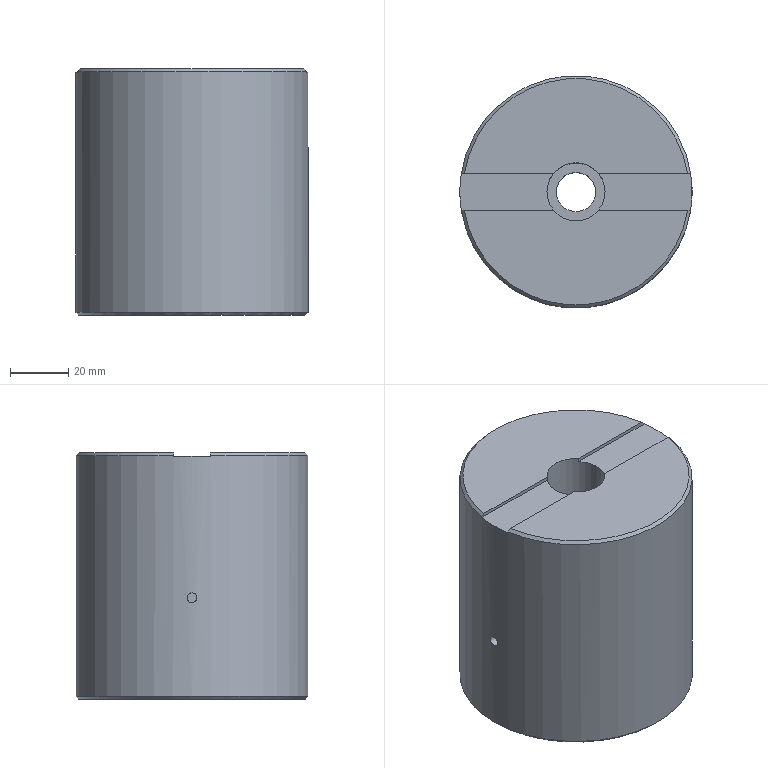Part | STEP file | 008_id4122_x_t | 1 solid | 18 faces | box 80 x 80 x 85 mm | volume 404311 mm3 | plane 11 | cylinder 4 | cone 3 | commonest cylinder face diameters 3.4 x1 13.509 x1 20.008 x1 80 x1
STEP:
#1=CARTESIAN_POINT('',(2359.705,-548.65,5.));
#2=VERTEX_POINT('',#1);
#3=CARTESIAN_POINT('',(2328.956,-548.65,5.));
#4=VERTEX_POINT('',#3);
#5=CARTESIAN_POINT('',(2415.936,-548.65,5.));
#6=DIRECTION('',(-1.,0.,0.));
#7=VECTOR('',#6,1.);
#8=LINE('',#5,#7);
#9=EDGE_CURVE('',#2,#4,#8,.T.);
#10=ORIENTED_EDGE('',*,*,#9,.F.);
#11=CARTESIAN_POINT('',(2375.166,-548.65,5.));
#12=VERTEX_POINT('',#11);
#13=CARTESIAN_POINT('',(2367.435,-555.,5.));
#14=DIRECTION('',(0.,0.,-1.));
#15=DIRECTION('',(1.,0.,0.));
#16=AXIS2_PLACEMENT_3D('',#13,#14,#15);
#17=CIRCLE('',#16,10.004);
#18=EDGE_CURVE('',#2,#12,#17,.T.);
#19=ORIENTED_EDGE('',*,*,#18,.T.);
#20=CARTESIAN_POINT('',(2405.915,-548.65,5.));
#21=VERTEX_POINT('',#20);
#22=CARTESIAN_POINT('',(2415.936,-548.65,5.));
#23=DIRECTION('',(-1.,0.,0.));
#24=VECTOR('',#23,1.);
#25=LINE('',#22,#24);
#26=EDGE_CURVE('',#21,#12,#25,.T.);
#27=ORIENTED_EDGE('',*,*,#26,.F.);
#28=CARTESIAN_POINT('',(2367.435,-555.,5.));
#29=DIRECTION('',(0.,0.,-1.));
#30=DIRECTION('',(-1.,0.,0.));
#31=AXIS2_PLACEMENT_3D('',#28,#29,#30);
#32=CIRCLE('',#31,39.);
#33=EDGE_CURVE('',#4,#21,#32,.T.);
#34=ORIENTED_EDGE('',*,*,#33,.F.);
#35=EDGE_LOOP('',(#10,#19,#27,#34));
#36=FACE_OUTER_BOUND('',#35,.T.);
#37=CARTESIAN_POINT('',(2367.435,-555.,5.));
#38=DIRECTION('',(0.,0.,1.));
#39=DIRECTION('',(-1.,0.,0.));
#40=AXIS2_PLACEMENT_3D('',#37,#38,#39);
#41=PLANE('',#40);
#42=ADVANCED_FACE('',(#36),#41,.T.);
#43=CARTESIAN_POINT('',(2405.915,-561.35,5.));
#44=VERTEX_POINT('',#43);
#45=CARTESIAN_POINT('',(2375.166,-561.35,5.));
#46=VERTEX_POINT('',#45);
#47=CARTESIAN_POINT('',(2415.936,-561.35,5.));
#48=DIRECTION('',(-1.,0.,0.));
#49=VECTOR('',#48,1.);
#50=LINE('',#47,#49);
#51=EDGE_CURVE('',#44,#46,#50,.T.);
#52=ORIENTED_EDGE('',*,*,#51,.T.);
#53=CARTESIAN_POINT('',(2359.705,-561.35,5.));
#54=VERTEX_POINT('',#53);
#55=CARTESIAN_POINT('',(2367.435,-555.,5.));
#56=DIRECTION('',(0.,0.,-1.));
#57=DIRECTION('',(1.,0.,0.));
#58=AXIS2_PLACEMENT_3D('',#55,#56,#57);
#59=CIRCLE('',#58,10.004);
#60=EDGE_CURVE('',#46,#54,#59,.T.);
#61=ORIENTED_EDGE('',*,*,#60,.T.);
#62=CARTESIAN_POINT('',(2328.956,-561.35,5.));
#63=VERTEX_POINT('',#62);
#64=CARTESIAN_POINT('',(2415.936,-561.35,5.));
#65=DIRECTION('',(-1.,0.,0.));
#66=VECTOR('',#65,1.);
#67=LINE('',#64,#66);
#68=EDGE_CURVE('',#54,#63,#67,.T.);
#69=ORIENTED_EDGE('',*,*,#68,.T.);
#70=CARTESIAN_POINT('',(2367.435,-555.,5.));
#71=DIRECTION('',(0.,0.,-1.));
#72=DIRECTION('',(-1.,0.,0.));
#73=AXIS2_PLACEMENT_3D('',#70,#71,#72);
#74=CIRCLE('',#73,39.);
#75=EDGE_CURVE('',#44,#63,#74,.T.);
#76=ORIENTED_EDGE('',*,*,#75,.F.);
#77=EDGE_LOOP('',(#52,#61,#69,#76));
#78=FACE_OUTER_BOUND('',#77,.T.);
#79=CARTESIAN_POINT('',(2367.435,-555.,5.));
#80=DIRECTION('',(0.,0.,1.));
#81=DIRECTION('',(-1.,0.,0.));
#82=AXIS2_PLACEMENT_3D('',#79,#80,#81);
#83=PLANE('',#82);
#84=ADVANCED_FACE('',(#78),#83,.T.);
#85=CARTESIAN_POINT('',(2327.435,-555.,-79.));
#86=VERTEX_POINT('',#85);
#87=CARTESIAN_POINT('',(2367.435,-555.,-79.));
#88=DIRECTION('',(0.,0.,-1.));
#89=DIRECTION('',(-1.,0.,0.));
#90=AXIS2_PLACEMENT_3D('',#87,#88,#89);
#91=CIRCLE('',#90,40.);
#92=EDGE_CURVE('',#86,#86,#91,.T.);
#93=ORIENTED_EDGE('',*,*,#92,.F.);
#94=EDGE_LOOP('',(#93));
#95=FACE_BOUND('',#94,.T.);
#96=CARTESIAN_POINT('',(2406.928,-548.65,3.73));
#97=VERTEX_POINT('',#96);
#98=CARTESIAN_POINT('',(2406.928,-548.65,4.));
#99=VERTEX_POINT('',#98);
#100=CARTESIAN_POINT('',(2406.928,-548.65,-80.));
#101=DIRECTION('',(0.,0.,1.));
#102=VECTOR('',#101,1.);
#103=LINE('',#100,#102);
#104=EDGE_CURVE('',#97,#99,#103,.T.);
#105=ORIENTED_EDGE('',*,*,#104,.F.);
#106=CARTESIAN_POINT('',(2406.928,-561.35,3.73));
#107=VERTEX_POINT('',#106);
#108=CARTESIAN_POINT('',(2367.435,-555.,3.73));
#109=DIRECTION('',(0.,0.,1.));
#110=DIRECTION('',(0.,-1.,0.));
#111=AXIS2_PLACEMENT_3D('',#108,#109,#110);
#112=CIRCLE('',#111,40.);
#113=EDGE_CURVE('',#107,#97,#112,.T.);
#114=ORIENTED_EDGE('',*,*,#113,.F.);
#115=CARTESIAN_POINT('',(2406.928,-561.35,4.));
#116=VERTEX_POINT('',#115);
#117=CARTESIAN_POINT('',(2406.928,-561.35,-80.));
#118=DIRECTION('',(0.,0.,-1.));
#119=VECTOR('',#118,1.);
#120=LINE('',#117,#119);
#121=EDGE_CURVE('',#116,#107,#120,.T.);
#122=ORIENTED_EDGE('',*,*,#121,.F.);
#123=CARTESIAN_POINT('',(2327.942,-561.35,4.));
#124=VERTEX_POINT('',#123);
#125=CARTESIAN_POINT('',(2367.435,-555.,4.));
#126=DIRECTION('',(0.,0.,1.));
#127=DIRECTION('',(-1.,0.,0.));
#128=AXIS2_PLACEMENT_3D('',#125,#126,#127);
#129=CIRCLE('',#128,40.);
#130=EDGE_CURVE('',#124,#116,#129,.T.);
#131=ORIENTED_EDGE('',*,*,#130,.F.);
#132=CARTESIAN_POINT('',(2327.942,-561.35,3.73));
#133=VERTEX_POINT('',#132);
#134=CARTESIAN_POINT('',(2327.942,-561.35,-80.));
#135=DIRECTION('',(0.,0.,1.));
#136=VECTOR('',#135,1.);
#137=LINE('',#134,#136);
#138=EDGE_CURVE('',#133,#124,#137,.T.);
#139=ORIENTED_EDGE('',*,*,#138,.F.);
#140=CARTESIAN_POINT('',(2327.942,-548.65,3.73));
#141=VERTEX_POINT('',#140);
#142=CARTESIAN_POINT('',(2367.435,-555.,3.73));
#143=DIRECTION('',(0.,0.,1.));
#144=DIRECTION('',(0.,-1.,0.));
#145=AXIS2_PLACEMENT_3D('',#142,#143,#144);
#146=CIRCLE('',#145,40.);
#147=EDGE_CURVE('',#141,#133,#146,.T.);
#148=ORIENTED_EDGE('',*,*,#147,.F.);
#149=CARTESIAN_POINT('',(2327.942,-548.65,4.));
#150=VERTEX_POINT('',#149);
#151=CARTESIAN_POINT('',(2327.942,-548.65,-80.));
#152=DIRECTION('',(0.,0.,-1.));
#153=VECTOR('',#152,1.);
#154=LINE('',#151,#153);
#155=EDGE_CURVE('',#150,#141,#154,.T.);
#156=ORIENTED_EDGE('',*,*,#155,.F.);
#157=CARTESIAN_POINT('',(2367.435,-555.,4.));
#158=DIRECTION('',(0.,0.,1.));
#159=DIRECTION('',(-1.,0.,0.));
#160=AXIS2_PLACEMENT_3D('',#157,#158,#159);
#161=CIRCLE('',#160,40.);
#162=EDGE_CURVE('',#99,#150,#161,.T.);
#163=ORIENTED_EDGE('',*,*,#162,.F.);
#164=EDGE_LOOP('',(#105,#114,#122,#131,#139,#148,#156,#163));
#165=FACE_BOUND('',#164,.T.);
#166=CARTESIAN_POINT('',(2327.436,-555.182,-43.31));
#167=VERTEX_POINT('',#166);
#168=CARTESIAN_POINT('',(2327.436,-555.182,-43.31));
#169=CARTESIAN_POINT('',(2327.435,-554.993,-43.289));
#170=CARTESIAN_POINT('',(2327.435,-554.798,-43.301));
#171=CARTESIAN_POINT('',(2327.437,-554.613,-43.345));
#172=CARTESIAN_POINT('',(2327.439,-554.427,-43.388));
#173=CARTESIAN_POINT('',(2327.442,-554.247,-43.464));
#174=CARTESIAN_POINT('',(2327.446,-554.087,-43.566));
#175=CARTESIAN_POINT('',(2327.449,-553.926,-43.668));
#176=CARTESIAN_POINT('',(2327.454,-553.781,-43.799));
#177=CARTESIAN_POINT('',(2327.458,-553.664,-43.949));
#178=CARTESIAN_POINT('',(2327.461,-553.546,-44.099));
#179=CARTESIAN_POINT('',(2327.465,-553.453,-44.271));
#180=CARTESIAN_POINT('',(2327.468,-553.391,-44.451));
#181=CARTESIAN_POINT('',(2327.47,-553.33,-44.631));
#182=CARTESIAN_POINT('',(2327.471,-553.298,-44.824));
#183=CARTESIAN_POINT('',(2327.471,-553.3,-45.014));
#184=CARTESIAN_POINT('',(2327.471,-553.302,-45.204));
#185=CARTESIAN_POINT('',(2327.47,-553.336,-45.397));
#186=CARTESIAN_POINT('',(2327.467,-553.4,-45.576));
#187=CARTESIAN_POINT('',(2327.465,-553.465,-45.755));
#188=CARTESIAN_POINT('',(2327.461,-553.561,-45.925));
#189=CARTESIAN_POINT('',(2327.457,-553.681,-46.072));
#190=CARTESIAN_POINT('',(2327.453,-553.801,-46.22));
#191=CARTESIAN_POINT('',(2327.449,-553.948,-46.349));
#192=CARTESIAN_POINT('',(2327.445,-554.11,-46.448));
#193=CARTESIAN_POINT('',(2327.442,-554.272,-46.548));
#194=CARTESIAN_POINT('',(2327.439,-554.454,-46.621));
#195=CARTESIAN_POINT('',(2327.437,-554.64,-46.661));
#196=CARTESIAN_POINT('',(2327.435,-554.826,-46.702));
#197=CARTESIAN_POINT('',(2327.435,-555.021,-46.71));
#198=CARTESIAN_POINT('',(2327.436,-555.21,-46.687));
#199=CARTESIAN_POINT('',(2327.437,-555.399,-46.664));
#200=CARTESIAN_POINT('',(2327.439,-555.586,-46.607));
#201=CARTESIAN_POINT('',(2327.442,-555.756,-46.523));
#202=CARTESIAN_POINT('',(2327.446,-555.926,-46.438));
#203=CARTESIAN_POINT('',(2327.45,-556.084,-46.323));
#204=CARTESIAN_POINT('',(2327.454,-556.217,-46.187));
#205=CARTESIAN_POINT('',(2327.458,-556.35,-46.051));
#206=CARTESIAN_POINT('',(2327.462,-556.461,-45.89));
#207=CARTESIAN_POINT('',(2327.465,-556.541,-45.717));
#208=CARTESIAN_POINT('',(2327.468,-556.622,-45.545));
#209=CARTESIAN_POINT('',(2327.47,-556.673,-45.356));
#210=CARTESIAN_POINT('',(2327.471,-556.692,-45.166));
#211=CARTESIAN_POINT('',(2327.472,-556.71,-44.977));
#212=CARTESIAN_POINT('',(2327.471,-556.697,-44.782));
#213=CARTESIAN_POINT('',(2327.469,-556.652,-44.597));
#214=CARTESIAN_POINT('',(2327.467,-556.607,-44.413));
#215=CARTESIAN_POINT('',(2327.464,-556.529,-44.233));
#216=CARTESIAN_POINT('',(2327.461,-556.425,-44.074));
#217=CARTESIAN_POINT('',(2327.457,-556.322,-43.914));
#218=CARTESIAN_POINT('',(2327.453,-556.189,-43.77));
#219=CARTESIAN_POINT('',(2327.449,-556.039,-43.654));
#220=CARTESIAN_POINT('',(2327.445,-555.888,-43.538));
#221=CARTESIAN_POINT('',(2327.441,-555.715,-43.446));
#222=CARTESIAN_POINT('',(2327.439,-555.535,-43.386));
#223=CARTESIAN_POINT('',(2327.437,-555.42,-43.348));
#224=CARTESIAN_POINT('',(2327.436,-555.301,-43.323));
#225=CARTESIAN_POINT('',(2327.436,-555.182,-43.31));
#226=B_SPLINE_CURVE_WITH_KNOTS('',3,(#168,#169,#170,#171,#172,#173,#174,#175,#176,#177,#178,#179,#180,#181,#182,#183,#184,#185,#186,#187,#188,#189,#190,#191,#192,#193,#194,#195,#196,#197,#198,#199,#200,#201,#202,#203,#204,#205,#206,#207,#208,#209,#210,#211,#212,#213,#214,#215,#216,#217,#218,#219,#220,#221,#222,#223,#224,#225),.UNSPECIFIED.,.T.,.F.,(1,3,3,3,3,3,3,3,3,3,3,3,3,3,3,3,3,3,3,3,3,1),(-0.03366,0.,0.05366,0.1073,0.161,0.2147,0.2684,0.3221,0.3757,0.4295,0.4832,0.5369,0.5905,0.6442,0.6979,0.7516,0.8053,0.8589,0.9126,0.9663,1.,1.054),.UNSPECIFIED.);
#227=EDGE_CURVE('',#167,#167,#226,.T.);
#228=ORIENTED_EDGE('',*,*,#227,.F.);
#229=EDGE_LOOP('',(#228));
#230=FACE_BOUND('',#229,.T.);
#231=CARTESIAN_POINT('',(2367.435,-555.,-80.));
#232=DIRECTION('',(0.,0.,1.));
#233=DIRECTION('',(-1.,0.,0.));
#234=AXIS2_PLACEMENT_3D('',#231,#232,#233);
#235=CYLINDRICAL_SURFACE('',#234,40.);
#236=ADVANCED_FACE('',(#95,#165,#230),#235,.T.);
#237=CARTESIAN_POINT('',(2374.19,-555.,-80.));
#238=VERTEX_POINT('',#237);
#239=CARTESIAN_POINT('',(2367.435,-555.,-80.));
#240=DIRECTION('',(0.,0.,1.));
#241=DIRECTION('',(1.,0.,0.));
#242=AXIS2_PLACEMENT_3D('',#239,#240,#241);
#243=CIRCLE('',#242,6.755);
#244=EDGE_CURVE('',#238,#238,#243,.T.);
#245=ORIENTED_EDGE('',*,*,#244,.T.);
#246=EDGE_LOOP('',(#245));
#247=FACE_BOUND('',#246,.T.);
#248=CARTESIAN_POINT('',(2328.435,-555.,-80.));
#249=VERTEX_POINT('',#248);
#250=CARTESIAN_POINT('',(2367.435,-555.,-80.));
#251=DIRECTION('',(0.,0.,1.));
#252=DIRECTION('',(-1.,0.,0.));
#253=AXIS2_PLACEMENT_3D('',#250,#251,#252);
#254=CIRCLE('',#253,39.);
#255=EDGE_CURVE('',#249,#249,#254,.T.);
#256=ORIENTED_EDGE('',*,*,#255,.F.);
#257=EDGE_LOOP('',(#256));
#258=FACE_BOUND('',#257,.T.);
#259=CARTESIAN_POINT('',(2367.435,-555.,-80.));
#260=DIRECTION('',(0.,0.,1.));
#261=DIRECTION('',(-1.,0.,0.));
#262=AXIS2_PLACEMENT_3D('',#259,#260,#261);
#263=PLANE('',#262);
#264=ADVANCED_FACE('',(#247,#258),#263,.F.);
#265=CARTESIAN_POINT('',(2375.166,-548.65,3.73));
#266=VERTEX_POINT('',#265);
#267=CARTESIAN_POINT('',(2375.166,-548.65,5.));
#268=DIRECTION('',(0.,0.,1.));
#269=VECTOR('',#268,1.);
#270=LINE('',#267,#269);
#271=EDGE_CURVE('',#266,#12,#270,.T.);
#272=ORIENTED_EDGE('',*,*,#271,.F.);
#273=CARTESIAN_POINT('',(2415.936,-548.65,3.73));
#274=DIRECTION('',(-1.,0.,0.));
#275=VECTOR('',#274,1.);
#276=LINE('',#273,#275);
#277=EDGE_CURVE('',#97,#266,#276,.T.);
#278=ORIENTED_EDGE('',*,*,#277,.F.);
#279=ORIENTED_EDGE('',*,*,#104,.T.);
#280=CARTESIAN_POINT('',(2405.915,-548.65,5.));
#281=CARTESIAN_POINT('',(2406.253,-548.65,4.667));
#282=CARTESIAN_POINT('',(2406.59,-548.65,4.333));
#283=CARTESIAN_POINT('',(2406.928,-548.65,4.));
#284=B_SPLINE_CURVE_WITH_KNOTS('',3,(#280,#281,#282,#283),.UNSPECIFIED.,.F.,.F.,(4,4),(0.,1.),.UNSPECIFIED.);
#285=EDGE_CURVE('',#21,#99,#284,.T.);
#286=ORIENTED_EDGE('',*,*,#285,.F.);
#287=ORIENTED_EDGE('',*,*,#26,.T.);
#288=EDGE_LOOP('',(#272,#278,#279,#286,#287));
#289=FACE_OUTER_BOUND('',#288,.T.);
#290=CARTESIAN_POINT('',(2415.936,-548.65,5.));
#291=DIRECTION('',(0.,-1.,0.));
#292=DIRECTION('',(0.,0.,-1.));
#293=AXIS2_PLACEMENT_3D('',#290,#291,#292);
#294=PLANE('',#293);
#295=ADVANCED_FACE('',(#289),#294,.T.);
#296=CARTESIAN_POINT('',(2375.166,-561.35,3.73));
#297=VERTEX_POINT('',#296);
#298=CARTESIAN_POINT('',(2367.435,-555.,3.73));
#299=DIRECTION('',(0.,0.,1.));
#300=DIRECTION('',(0.,-1.,0.));
#301=AXIS2_PLACEMENT_3D('',#298,#299,#300);
#302=CIRCLE('',#301,10.004);
#303=EDGE_CURVE('',#297,#266,#302,.T.);
#304=ORIENTED_EDGE('',*,*,#303,.F.);
#305=CARTESIAN_POINT('',(2415.936,-561.35,3.73));
#306=DIRECTION('',(-1.,0.,0.));
#307=VECTOR('',#306,1.);
#308=LINE('',#305,#307);
#309=EDGE_CURVE('',#107,#297,#308,.T.);
#310=ORIENTED_EDGE('',*,*,#309,.F.);
#311=ORIENTED_EDGE('',*,*,#113,.T.);
#312=ORIENTED_EDGE('',*,*,#277,.T.);
#313=EDGE_LOOP('',(#304,#310,#311,#312));
#314=FACE_OUTER_BOUND('',#313,.T.);
#315=CARTESIAN_POINT('',(2415.936,-548.65,3.73));
#316=DIRECTION('',(0.,0.,1.));
#317=DIRECTION('',(0.,-1.,0.));
#318=AXIS2_PLACEMENT_3D('',#315,#316,#317);
#319=PLANE('',#318);
#320=ADVANCED_FACE('',(#314),#319,.T.);
#321=CARTESIAN_POINT('',(2375.166,-561.35,5.));
#322=DIRECTION('',(0.,0.,-1.));
#323=VECTOR('',#322,1.);
#324=LINE('',#321,#323);
#325=EDGE_CURVE('',#46,#297,#324,.T.);
#326=ORIENTED_EDGE('',*,*,#325,.F.);
#327=ORIENTED_EDGE('',*,*,#51,.F.);
#328=CARTESIAN_POINT('',(2406.928,-561.35,4.));
#329=CARTESIAN_POINT('',(2406.59,-561.35,4.333));
#330=CARTESIAN_POINT('',(2406.253,-561.35,4.667));
#331=CARTESIAN_POINT('',(2405.915,-561.35,5.));
#332=B_SPLINE_CURVE_WITH_KNOTS('',3,(#328,#329,#330,#331),.UNSPECIFIED.,.F.,.F.,(4,4),(0.,1.),.UNSPECIFIED.);
#333=EDGE_CURVE('',#116,#44,#332,.T.);
#334=ORIENTED_EDGE('',*,*,#333,.F.);
#335=ORIENTED_EDGE('',*,*,#121,.T.);
#336=ORIENTED_EDGE('',*,*,#309,.T.);
#337=EDGE_LOOP('',(#326,#327,#334,#335,#336));
#338=FACE_OUTER_BOUND('',#337,.T.);
#339=CARTESIAN_POINT('',(2415.936,-561.35,3.73));
#340=DIRECTION('',(0.,1.,0.));
#341=DIRECTION('',(0.,0.,1.));
#342=AXIS2_PLACEMENT_3D('',#339,#340,#341);
#343=PLANE('',#342);
#344=ADVANCED_FACE('',(#338),#343,.T.);
#345=CARTESIAN_POINT('',(2359.705,-548.65,3.73));
#346=VERTEX_POINT('',#345);
#347=CARTESIAN_POINT('',(2359.705,-561.35,3.73));
#348=VERTEX_POINT('',#347);
#349=CARTESIAN_POINT('',(2367.435,-555.,3.73));
#350=DIRECTION('',(0.,0.,1.));
#351=DIRECTION('',(0.,-1.,0.));
#352=AXIS2_PLACEMENT_3D('',#349,#350,#351);
#353=CIRCLE('',#352,10.004);
#354=EDGE_CURVE('',#346,#348,#353,.T.);
#355=ORIENTED_EDGE('',*,*,#354,.F.);
#356=CARTESIAN_POINT('',(2415.936,-548.65,3.73));
#357=DIRECTION('',(-1.,0.,0.));
#358=VECTOR('',#357,1.);
#359=LINE('',#356,#358);
#360=EDGE_CURVE('',#346,#141,#359,.T.);
#361=ORIENTED_EDGE('',*,*,#360,.T.);
#362=ORIENTED_EDGE('',*,*,#147,.T.);
#363=CARTESIAN_POINT('',(2415.936,-561.35,3.73));
#364=DIRECTION('',(-1.,0.,0.));
#365=VECTOR('',#364,1.);
#366=LINE('',#363,#365);
#367=EDGE_CURVE('',#348,#133,#366,.T.);
#368=ORIENTED_EDGE('',*,*,#367,.F.);
#369=EDGE_LOOP('',(#355,#361,#362,#368));
#370=FACE_OUTER_BOUND('',#369,.T.);
#371=CARTESIAN_POINT('',(2415.936,-548.65,3.73));
#372=DIRECTION('',(0.,0.,1.));
#373=DIRECTION('',(0.,-1.,0.));
#374=AXIS2_PLACEMENT_3D('',#371,#372,#373);
#375=PLANE('',#374);
#376=ADVANCED_FACE('',(#370),#375,.T.);
#377=CARTESIAN_POINT('',(2359.705,-548.65,5.));
#378=DIRECTION('',(0.,0.,-1.));
#379=VECTOR('',#378,1.);
#380=LINE('',#377,#379);
#381=EDGE_CURVE('',#2,#346,#380,.T.);
#382=ORIENTED_EDGE('',*,*,#381,.F.);
#383=ORIENTED_EDGE('',*,*,#9,.T.);
#384=CARTESIAN_POINT('',(2327.942,-548.65,4.));
#385=CARTESIAN_POINT('',(2328.28,-548.65,4.333));
#386=CARTESIAN_POINT('',(2328.618,-548.65,4.667));
#387=CARTESIAN_POINT('',(2328.956,-548.65,5.));
#388=B_SPLINE_CURVE_WITH_KNOTS('',3,(#384,#385,#386,#387),.UNSPECIFIED.,.F.,.F.,(4,4),(0.,1.),.UNSPECIFIED.);
#389=EDGE_CURVE('',#150,#4,#388,.T.);
#390=ORIENTED_EDGE('',*,*,#389,.F.);
#391=ORIENTED_EDGE('',*,*,#155,.T.);
#392=ORIENTED_EDGE('',*,*,#360,.F.);
#393=EDGE_LOOP('',(#382,#383,#390,#391,#392));
#394=FACE_OUTER_BOUND('',#393,.T.);
#395=CARTESIAN_POINT('',(2415.936,-548.65,5.));
#396=DIRECTION('',(0.,-1.,0.));
#397=DIRECTION('',(0.,0.,-1.));
#398=AXIS2_PLACEMENT_3D('',#395,#396,#397);
#399=PLANE('',#398);
#400=ADVANCED_FACE('',(#394),#399,.T.);
#401=CARTESIAN_POINT('',(2359.705,-561.35,5.));
#402=DIRECTION('',(0.,0.,1.));
#403=VECTOR('',#402,1.);
#404=LINE('',#401,#403);
#405=EDGE_CURVE('',#348,#54,#404,.T.);
#406=ORIENTED_EDGE('',*,*,#405,.F.);
#407=ORIENTED_EDGE('',*,*,#367,.T.);
#408=ORIENTED_EDGE('',*,*,#138,.T.);
#409=CARTESIAN_POINT('',(2328.956,-561.35,5.));
#410=CARTESIAN_POINT('',(2328.618,-561.35,4.667));
#411=CARTESIAN_POINT('',(2328.28,-561.35,4.333));
#412=CARTESIAN_POINT('',(2327.942,-561.35,4.));
#413=B_SPLINE_CURVE_WITH_KNOTS('',3,(#409,#410,#411,#412),.UNSPECIFIED.,.F.,.F.,(4,4),(0.,1.),.UNSPECIFIED.);
#414=EDGE_CURVE('',#63,#124,#413,.T.);
#415=ORIENTED_EDGE('',*,*,#414,.F.);
#416=ORIENTED_EDGE('',*,*,#68,.F.);
#417=EDGE_LOOP('',(#406,#407,#408,#415,#416));
#418=FACE_OUTER_BOUND('',#417,.T.);
#419=CARTESIAN_POINT('',(2415.936,-561.35,3.73));
#420=DIRECTION('',(0.,1.,0.));
#421=DIRECTION('',(0.,0.,1.));
#422=AXIS2_PLACEMENT_3D('',#419,#420,#421);
#423=PLANE('',#422);
#424=ADVANCED_FACE('',(#418),#423,.T.);
#425=ORIENTED_EDGE('',*,*,#227,.T.);
#426=EDGE_LOOP('',(#425));
#427=FACE_BOUND('',#426,.T.);
#428=CARTESIAN_POINT('',(2341.936,-556.7,-45.));
#429=VERTEX_POINT('',#428);
#430=CARTESIAN_POINT('',(2341.936,-555.,-45.));
#431=DIRECTION('',(1.,0.,0.));
#432=DIRECTION('',(0.,-1.,0.));
#433=AXIS2_PLACEMENT_3D('',#430,#431,#432);
#434=CIRCLE('',#433,1.7);
#435=EDGE_CURVE('',#429,#429,#434,.T.);
#436=ORIENTED_EDGE('',*,*,#435,.T.);
#437=EDGE_LOOP('',(#436));
#438=FACE_BOUND('',#437,.T.);
#439=CARTESIAN_POINT('',(2341.936,-555.,-45.));
#440=DIRECTION('',(-1.,0.,0.));
#441=DIRECTION('',(0.,1.,0.));
#442=AXIS2_PLACEMENT_3D('',#439,#440,#441);
#443=CYLINDRICAL_SURFACE('',#442,1.7);
#444=ADVANCED_FACE('',(#427,#438),#443,.F.);
#445=ORIENTED_EDGE('',*,*,#435,.F.);
#446=EDGE_LOOP('',(#445));
#447=FACE_OUTER_BOUND('',#446,.T.);
#448=CARTESIAN_POINT('',(2341.936,-555.,-45.));
#449=DIRECTION('',(1.,0.,0.));
#450=DIRECTION('',(0.,-1.,0.));
#451=AXIS2_PLACEMENT_3D('',#448,#449,#450);
#452=PLANE('',#451);
#453=ADVANCED_FACE('',(#447),#452,.F.);
#454=ORIENTED_EDGE('',*,*,#389,.T.);
#455=ORIENTED_EDGE('',*,*,#33,.T.);
#456=ORIENTED_EDGE('',*,*,#285,.T.);
#457=ORIENTED_EDGE('',*,*,#162,.T.);
#458=EDGE_LOOP('',(#454,#455,#456,#457));
#459=FACE_OUTER_BOUND('',#458,.T.);
#460=CARTESIAN_POINT('',(2367.435,-555.,5.));
#461=DIRECTION('',(0.,0.,-1.));
#462=DIRECTION('',(1.,0.,0.));
#463=AXIS2_PLACEMENT_3D('',#460,#461,#462);
#464=CONICAL_SURFACE('',#463,39.,45.);
#465=ADVANCED_FACE('',(#459),#464,.T.);
#466=ORIENTED_EDGE('',*,*,#333,.T.);
#467=ORIENTED_EDGE('',*,*,#75,.T.);
#468=ORIENTED_EDGE('',*,*,#414,.T.);
#469=ORIENTED_EDGE('',*,*,#130,.T.);
#470=EDGE_LOOP('',(#466,#467,#468,#469));
#471=FACE_OUTER_BOUND('',#470,.T.);
#472=CARTESIAN_POINT('',(2367.435,-555.,5.));
#473=DIRECTION('',(0.,0.,-1.));
#474=DIRECTION('',(1.,0.,0.));
#475=AXIS2_PLACEMENT_3D('',#472,#473,#474);
#476=CONICAL_SURFACE('',#475,39.,45.);
#477=ADVANCED_FACE('',(#471),#476,.T.);
#478=ORIENTED_EDGE('',*,*,#255,.T.);
#479=EDGE_LOOP('',(#478));
#480=FACE_BOUND('',#479,.T.);
#481=ORIENTED_EDGE('',*,*,#92,.T.);
#482=EDGE_LOOP('',(#481));
#483=FACE_BOUND('',#482,.T.);
#484=CARTESIAN_POINT('',(2367.435,-555.,-79.));
#485=DIRECTION('',(0.,0.,1.));
#486=DIRECTION('',(-1.,0.,0.));
#487=AXIS2_PLACEMENT_3D('',#484,#485,#486);
#488=CONICAL_SURFACE('',#487,40.,45.);
#489=ADVANCED_FACE('',(#480,#483),#488,.T.);
#490=CARTESIAN_POINT('',(2360.681,-555.,-50.));
#491=VERTEX_POINT('',#490);
#492=CARTESIAN_POINT('',(2367.435,-555.,-50.));
#493=DIRECTION('',(0.,0.,-1.));
#494=DIRECTION('',(-1.,0.,0.));
#495=AXIS2_PLACEMENT_3D('',#492,#493,#494);
#496=CIRCLE('',#495,6.755);
#497=EDGE_CURVE('',#491,#491,#496,.T.);
#498=ORIENTED_EDGE('',*,*,#497,.F.);
#499=EDGE_LOOP('',(#498));
#500=FACE_BOUND('',#499,.T.);
#501=ORIENTED_EDGE('',*,*,#244,.F.);
#502=EDGE_LOOP('',(#501));
#503=FACE_BOUND('',#502,.T.);
#504=CARTESIAN_POINT('',(2367.435,-555.,5.));
#505=DIRECTION('',(0.,0.,-1.));
#506=DIRECTION('',(1.,0.,0.));
#507=AXIS2_PLACEMENT_3D('',#504,#505,#506);
#508=CYLINDRICAL_SURFACE('',#507,6.755);
#509=ADVANCED_FACE('',(#500,#503),#508,.F.);
#510=ORIENTED_EDGE('',*,*,#497,.T.);
#511=EDGE_LOOP('',(#510));
#512=FACE_BOUND('',#511,.T.);
#513=CARTESIAN_POINT('',(2377.439,-555.,-50.));
#514=VERTEX_POINT('',#513);
#515=CARTESIAN_POINT('',(2367.435,-555.,-50.));
#516=DIRECTION('',(0.,0.,-1.));
#517=DIRECTION('',(1.,0.,0.));
#518=AXIS2_PLACEMENT_3D('',#515,#516,#517);
#519=CIRCLE('',#518,10.004);
#520=EDGE_CURVE('',#514,#514,#519,.T.);
#521=ORIENTED_EDGE('',*,*,#520,.F.);
#522=EDGE_LOOP('',(#521));
#523=FACE_BOUND('',#522,.T.);
#524=CARTESIAN_POINT('',(2367.435,-555.,-50.));
#525=DIRECTION('',(0.,0.,-1.));
#526=DIRECTION('',(-1.,0.,0.));
#527=AXIS2_PLACEMENT_3D('',#524,#525,#526);
#528=PLANE('',#527);
#529=ADVANCED_FACE('',(#512,#523),#528,.F.);
#530=ORIENTED_EDGE('',*,*,#271,.T.);
#531=ORIENTED_EDGE('',*,*,#18,.F.);
#532=ORIENTED_EDGE('',*,*,#381,.T.);
#533=ORIENTED_EDGE('',*,*,#354,.T.);
#534=ORIENTED_EDGE('',*,*,#405,.T.);
#535=ORIENTED_EDGE('',*,*,#60,.F.);
#536=ORIENTED_EDGE('',*,*,#325,.T.);
#537=ORIENTED_EDGE('',*,*,#303,.T.);
#538=EDGE_LOOP('',(#530,#531,#532,#533,#534,#535,#536,#537));
#539=FACE_BOUND('',#538,.T.);
#540=ORIENTED_EDGE('',*,*,#520,.T.);
#541=EDGE_LOOP('',(#540));
#542=FACE_BOUND('',#541,.T.);
#543=CARTESIAN_POINT('',(2367.435,-555.,5.));
#544=DIRECTION('',(0.,0.,-1.));
#545=DIRECTION('',(1.,0.,0.));
#546=AXIS2_PLACEMENT_3D('',#543,#544,#545);
#547=CYLINDRICAL_SURFACE('',#546,10.004);
#548=ADVANCED_FACE('',(#539,#542),#547,.F.);
#549=CLOSED_SHELL('',(#42,#84,#236,#264,#295,#320,#344,#376,#400,#424,#444,#453,#465,#477,#489,#509,#529,#548));
#550=MANIFOLD_SOLID_BREP('',#549);
#551=(LENGTH_UNIT()NAMED_UNIT(*)SI_UNIT(.MILLI.,.METRE.));
#552=UNCERTAINTY_MEASURE_WITH_UNIT(LENGTH_MEASURE(0.0508),#551,'','');
#553=(NAMED_UNIT(*)PLANE_ANGLE_UNIT()SI_UNIT($,.RADIAN.));
#554=PLANE_ANGLE_MEASURE_WITH_UNIT(PLANE_ANGLE_MEASURE(0.01745),#553);
#555=DIMENSIONAL_EXPONENTS(0.,0.,0.,0.,0.,0.,0.);
#556=(CONVERSION_BASED_UNIT('DEGREE',#554)NAMED_UNIT(#555)PLANE_ANGLE_UNIT());
#557=(NAMED_UNIT(*)SI_UNIT($,.STERADIAN.)SOLID_ANGLE_UNIT());
#558=(GEOMETRIC_REPRESENTATION_CONTEXT(3)GLOBAL_UNCERTAINTY_ASSIGNED_CONTEXT((#552))GLOBAL_UNIT_ASSIGNED_CONTEXT((#551,#556,#557))REPRESENTATION_CONTEXT('',''));
#559=ADVANCED_BREP_SHAPE_REPRESENTATION('',(#550),#558);